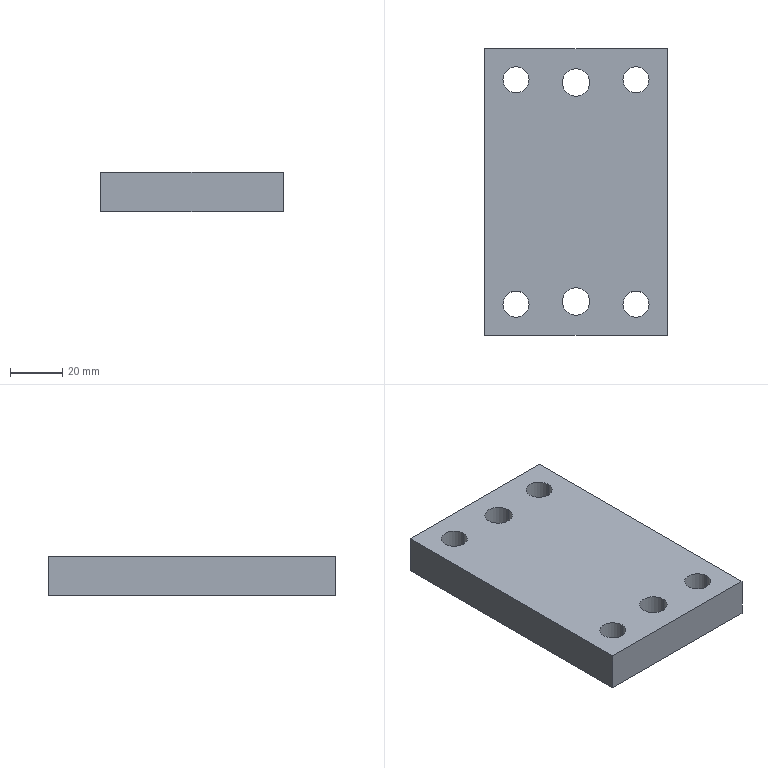Part | STEP file | Part 9^超升波生产线-2 | 1 solid | 18 faces | box 70 x 110 x 15 mm | volume 108190 mm3 | cylinder 12 | plane 6 | commonest cylinder face diameters 10 x8 10.5 x4
STEP:
#1=CARTESIAN_POINT('',(18.,-43.,15.));
#2=VERTEX_POINT('',#1);
#3=CARTESIAN_POINT('',(28.,-43.,15.));
#4=VERTEX_POINT('',#3);
#5=CARTESIAN_POINT('',(23.,-43.,15.));
#6=DIRECTION('',(0.,0.,1.));
#7=DIRECTION('',(1.,0.,0.));
#8=AXIS2_PLACEMENT_3D('',#5,#6,#7);
#9=CIRCLE('',#8,5.);
#10=EDGE_CURVE('',#2,#4,#9,.T.);
#11=ORIENTED_EDGE('',*,*,#10,.T.);
#12=CARTESIAN_POINT('',(28.,-43.,0.));
#13=VERTEX_POINT('',#12);
#14=CARTESIAN_POINT('',(28.,-43.,15.));
#15=DIRECTION('',(0.,0.,-1.));
#16=VECTOR('',#15,1000.);
#17=LINE('',#14,#16);
#18=EDGE_CURVE('',#4,#13,#17,.T.);
#19=ORIENTED_EDGE('',*,*,#18,.T.);
#20=CARTESIAN_POINT('',(18.,-43.,0.));
#21=VERTEX_POINT('',#20);
#22=CARTESIAN_POINT('',(23.,-43.,0.));
#23=DIRECTION('',(0.,0.,1.));
#24=DIRECTION('',(1.,0.,0.));
#25=AXIS2_PLACEMENT_3D('',#22,#23,#24);
#26=CIRCLE('',#25,5.);
#27=EDGE_CURVE('',#21,#13,#26,.T.);
#28=ORIENTED_EDGE('',*,*,#27,.F.);
#29=CARTESIAN_POINT('',(18.,-43.,15.));
#30=DIRECTION('',(0.,0.,-1.));
#31=VECTOR('',#30,1000.);
#32=LINE('',#29,#31);
#33=EDGE_CURVE('',#2,#21,#32,.T.);
#34=ORIENTED_EDGE('',*,*,#33,.F.);
#35=EDGE_LOOP('',(#11,#19,#28,#34));
#36=FACE_OUTER_BOUND('',#35,.T.);
#37=CARTESIAN_POINT('',(23.,-43.,15.));
#38=DIRECTION('',(0.,0.,-1.));
#39=DIRECTION('',(-1.,0.,0.));
#40=AXIS2_PLACEMENT_3D('',#37,#38,#39);
#41=CYLINDRICAL_SURFACE('',#40,5.);
#42=ADVANCED_FACE('',(#36),#41,.F.);
#43=CARTESIAN_POINT('',(-28.,-43.,15.));
#44=VERTEX_POINT('',#43);
#45=CARTESIAN_POINT('',(-18.,-43.,15.));
#46=VERTEX_POINT('',#45);
#47=CARTESIAN_POINT('',(-23.,-43.,15.));
#48=DIRECTION('',(0.,0.,1.));
#49=DIRECTION('',(1.,0.,0.));
#50=AXIS2_PLACEMENT_3D('',#47,#48,#49);
#51=CIRCLE('',#50,5.);
#52=EDGE_CURVE('',#44,#46,#51,.T.);
#53=ORIENTED_EDGE('',*,*,#52,.T.);
#54=CARTESIAN_POINT('',(-18.,-43.,0.));
#55=VERTEX_POINT('',#54);
#56=CARTESIAN_POINT('',(-18.,-43.,15.));
#57=DIRECTION('',(0.,0.,-1.));
#58=VECTOR('',#57,1000.);
#59=LINE('',#56,#58);
#60=EDGE_CURVE('',#46,#55,#59,.T.);
#61=ORIENTED_EDGE('',*,*,#60,.T.);
#62=CARTESIAN_POINT('',(-28.,-43.,0.));
#63=VERTEX_POINT('',#62);
#64=CARTESIAN_POINT('',(-23.,-43.,0.));
#65=DIRECTION('',(0.,0.,1.));
#66=DIRECTION('',(1.,0.,0.));
#67=AXIS2_PLACEMENT_3D('',#64,#65,#66);
#68=CIRCLE('',#67,5.);
#69=EDGE_CURVE('',#63,#55,#68,.T.);
#70=ORIENTED_EDGE('',*,*,#69,.F.);
#71=CARTESIAN_POINT('',(-28.,-43.,15.));
#72=DIRECTION('',(0.,0.,-1.));
#73=VECTOR('',#72,1000.);
#74=LINE('',#71,#73);
#75=EDGE_CURVE('',#44,#63,#74,.T.);
#76=ORIENTED_EDGE('',*,*,#75,.F.);
#77=EDGE_LOOP('',(#53,#61,#70,#76));
#78=FACE_OUTER_BOUND('',#77,.T.);
#79=CARTESIAN_POINT('',(-23.,-43.,15.));
#80=DIRECTION('',(0.,0.,-1.));
#81=DIRECTION('',(-1.,0.,0.));
#82=AXIS2_PLACEMENT_3D('',#79,#80,#81);
#83=CYLINDRICAL_SURFACE('',#82,5.);
#84=ADVANCED_FACE('',(#78),#83,.F.);
#85=CARTESIAN_POINT('',(18.,43.,15.));
#86=VERTEX_POINT('',#85);
#87=CARTESIAN_POINT('',(28.,43.,15.));
#88=VERTEX_POINT('',#87);
#89=CARTESIAN_POINT('',(23.,43.,15.));
#90=DIRECTION('',(0.,0.,1.));
#91=DIRECTION('',(1.,0.,0.));
#92=AXIS2_PLACEMENT_3D('',#89,#90,#91);
#93=CIRCLE('',#92,5.);
#94=EDGE_CURVE('',#86,#88,#93,.T.);
#95=ORIENTED_EDGE('',*,*,#94,.T.);
#96=CARTESIAN_POINT('',(28.,43.,0.));
#97=VERTEX_POINT('',#96);
#98=CARTESIAN_POINT('',(28.,43.,15.));
#99=DIRECTION('',(0.,0.,-1.));
#100=VECTOR('',#99,1000.);
#101=LINE('',#98,#100);
#102=EDGE_CURVE('',#88,#97,#101,.T.);
#103=ORIENTED_EDGE('',*,*,#102,.T.);
#104=CARTESIAN_POINT('',(18.,43.,0.));
#105=VERTEX_POINT('',#104);
#106=CARTESIAN_POINT('',(23.,43.,0.));
#107=DIRECTION('',(0.,0.,1.));
#108=DIRECTION('',(1.,0.,0.));
#109=AXIS2_PLACEMENT_3D('',#106,#107,#108);
#110=CIRCLE('',#109,5.);
#111=EDGE_CURVE('',#105,#97,#110,.T.);
#112=ORIENTED_EDGE('',*,*,#111,.F.);
#113=CARTESIAN_POINT('',(18.,43.,15.));
#114=DIRECTION('',(0.,0.,-1.));
#115=VECTOR('',#114,1000.);
#116=LINE('',#113,#115);
#117=EDGE_CURVE('',#86,#105,#116,.T.);
#118=ORIENTED_EDGE('',*,*,#117,.F.);
#119=EDGE_LOOP('',(#95,#103,#112,#118));
#120=FACE_OUTER_BOUND('',#119,.T.);
#121=CARTESIAN_POINT('',(23.,43.,15.));
#122=DIRECTION('',(0.,0.,-1.));
#123=DIRECTION('',(-1.,0.,0.));
#124=AXIS2_PLACEMENT_3D('',#121,#122,#123);
#125=CYLINDRICAL_SURFACE('',#124,5.);
#126=ADVANCED_FACE('',(#120),#125,.F.);
#127=CARTESIAN_POINT('',(-28.,43.,15.));
#128=VERTEX_POINT('',#127);
#129=CARTESIAN_POINT('',(-18.,43.,15.));
#130=VERTEX_POINT('',#129);
#131=CARTESIAN_POINT('',(-23.,43.,15.));
#132=DIRECTION('',(0.,0.,1.));
#133=DIRECTION('',(1.,0.,0.));
#134=AXIS2_PLACEMENT_3D('',#131,#132,#133);
#135=CIRCLE('',#134,5.);
#136=EDGE_CURVE('',#128,#130,#135,.T.);
#137=ORIENTED_EDGE('',*,*,#136,.T.);
#138=CARTESIAN_POINT('',(-18.,43.,0.));
#139=VERTEX_POINT('',#138);
#140=CARTESIAN_POINT('',(-18.,43.,15.));
#141=DIRECTION('',(0.,0.,-1.));
#142=VECTOR('',#141,1000.);
#143=LINE('',#140,#142);
#144=EDGE_CURVE('',#130,#139,#143,.T.);
#145=ORIENTED_EDGE('',*,*,#144,.T.);
#146=CARTESIAN_POINT('',(-28.,43.,0.));
#147=VERTEX_POINT('',#146);
#148=CARTESIAN_POINT('',(-23.,43.,0.));
#149=DIRECTION('',(0.,0.,1.));
#150=DIRECTION('',(1.,0.,0.));
#151=AXIS2_PLACEMENT_3D('',#148,#149,#150);
#152=CIRCLE('',#151,5.);
#153=EDGE_CURVE('',#147,#139,#152,.T.);
#154=ORIENTED_EDGE('',*,*,#153,.F.);
#155=CARTESIAN_POINT('',(-28.,43.,15.));
#156=DIRECTION('',(0.,0.,-1.));
#157=VECTOR('',#156,1000.);
#158=LINE('',#155,#157);
#159=EDGE_CURVE('',#128,#147,#158,.T.);
#160=ORIENTED_EDGE('',*,*,#159,.F.);
#161=EDGE_LOOP('',(#137,#145,#154,#160));
#162=FACE_OUTER_BOUND('',#161,.T.);
#163=CARTESIAN_POINT('',(-23.,43.,15.));
#164=DIRECTION('',(0.,0.,-1.));
#165=DIRECTION('',(-1.,0.,0.));
#166=AXIS2_PLACEMENT_3D('',#163,#164,#165);
#167=CYLINDRICAL_SURFACE('',#166,5.);
#168=ADVANCED_FACE('',(#162),#167,.F.);
#169=CARTESIAN_POINT('',(-5.25,-42.,15.));
#170=VERTEX_POINT('',#169);
#171=CARTESIAN_POINT('',(5.25,-42.,15.));
#172=VERTEX_POINT('',#171);
#173=CARTESIAN_POINT('',(0.,-42.,15.));
#174=DIRECTION('',(0.,0.,1.));
#175=DIRECTION('',(1.,0.,0.));
#176=AXIS2_PLACEMENT_3D('',#173,#174,#175);
#177=CIRCLE('',#176,5.25);
#178=EDGE_CURVE('',#170,#172,#177,.T.);
#179=ORIENTED_EDGE('',*,*,#178,.T.);
#180=CARTESIAN_POINT('',(5.25,-42.,0.));
#181=VERTEX_POINT('',#180);
#182=CARTESIAN_POINT('',(5.25,-42.,15.));
#183=DIRECTION('',(0.,0.,-1.));
#184=VECTOR('',#183,1000.);
#185=LINE('',#182,#184);
#186=EDGE_CURVE('',#172,#181,#185,.T.);
#187=ORIENTED_EDGE('',*,*,#186,.T.);
#188=CARTESIAN_POINT('',(-5.25,-42.,0.));
#189=VERTEX_POINT('',#188);
#190=CARTESIAN_POINT('',(0.,-42.,0.));
#191=DIRECTION('',(0.,0.,1.));
#192=DIRECTION('',(1.,0.,0.));
#193=AXIS2_PLACEMENT_3D('',#190,#191,#192);
#194=CIRCLE('',#193,5.25);
#195=EDGE_CURVE('',#189,#181,#194,.T.);
#196=ORIENTED_EDGE('',*,*,#195,.F.);
#197=CARTESIAN_POINT('',(-5.25,-42.,15.));
#198=DIRECTION('',(0.,0.,-1.));
#199=VECTOR('',#198,1000.);
#200=LINE('',#197,#199);
#201=EDGE_CURVE('',#170,#189,#200,.T.);
#202=ORIENTED_EDGE('',*,*,#201,.F.);
#203=EDGE_LOOP('',(#179,#187,#196,#202));
#204=FACE_OUTER_BOUND('',#203,.T.);
#205=CARTESIAN_POINT('',(0.,-42.,15.));
#206=DIRECTION('',(0.,0.,-1.));
#207=DIRECTION('',(-1.,0.,0.));
#208=AXIS2_PLACEMENT_3D('',#205,#206,#207);
#209=CYLINDRICAL_SURFACE('',#208,5.25);
#210=ADVANCED_FACE('',(#204),#209,.F.);
#211=CARTESIAN_POINT('',(-5.25,42.,15.));
#212=VERTEX_POINT('',#211);
#213=CARTESIAN_POINT('',(5.25,42.,15.));
#214=VERTEX_POINT('',#213);
#215=CARTESIAN_POINT('',(0.,42.,15.));
#216=DIRECTION('',(0.,0.,1.));
#217=DIRECTION('',(1.,0.,0.));
#218=AXIS2_PLACEMENT_3D('',#215,#216,#217);
#219=CIRCLE('',#218,5.25);
#220=EDGE_CURVE('',#212,#214,#219,.T.);
#221=ORIENTED_EDGE('',*,*,#220,.T.);
#222=CARTESIAN_POINT('',(5.25,42.,0.));
#223=VERTEX_POINT('',#222);
#224=CARTESIAN_POINT('',(5.25,42.,15.));
#225=DIRECTION('',(0.,0.,-1.));
#226=VECTOR('',#225,1000.);
#227=LINE('',#224,#226);
#228=EDGE_CURVE('',#214,#223,#227,.T.);
#229=ORIENTED_EDGE('',*,*,#228,.T.);
#230=CARTESIAN_POINT('',(-5.25,42.,0.));
#231=VERTEX_POINT('',#230);
#232=CARTESIAN_POINT('',(0.,42.,0.));
#233=DIRECTION('',(0.,0.,1.));
#234=DIRECTION('',(1.,0.,0.));
#235=AXIS2_PLACEMENT_3D('',#232,#233,#234);
#236=CIRCLE('',#235,5.25);
#237=EDGE_CURVE('',#231,#223,#236,.T.);
#238=ORIENTED_EDGE('',*,*,#237,.F.);
#239=CARTESIAN_POINT('',(-5.25,42.,15.));
#240=DIRECTION('',(0.,0.,-1.));
#241=VECTOR('',#240,1000.);
#242=LINE('',#239,#241);
#243=EDGE_CURVE('',#212,#231,#242,.T.);
#244=ORIENTED_EDGE('',*,*,#243,.F.);
#245=EDGE_LOOP('',(#221,#229,#238,#244));
#246=FACE_OUTER_BOUND('',#245,.T.);
#247=CARTESIAN_POINT('',(0.,42.,15.));
#248=DIRECTION('',(0.,0.,-1.));
#249=DIRECTION('',(-1.,0.,0.));
#250=AXIS2_PLACEMENT_3D('',#247,#248,#249);
#251=CYLINDRICAL_SURFACE('',#250,5.25);
#252=ADVANCED_FACE('',(#246),#251,.F.);
#253=ORIENTED_EDGE('',*,*,#52,.F.);
#254=CARTESIAN_POINT('',(-23.,-43.,15.));
#255=DIRECTION('',(0.,0.,1.));
#256=DIRECTION('',(1.,0.,0.));
#257=AXIS2_PLACEMENT_3D('',#254,#255,#256);
#258=CIRCLE('',#257,5.);
#259=EDGE_CURVE('',#46,#44,#258,.T.);
#260=ORIENTED_EDGE('',*,*,#259,.F.);
#261=EDGE_LOOP('',(#253,#260));
#262=FACE_BOUND('',#261,.T.);
#263=ORIENTED_EDGE('',*,*,#136,.F.);
#264=CARTESIAN_POINT('',(-23.,43.,15.));
#265=DIRECTION('',(0.,0.,1.));
#266=DIRECTION('',(1.,0.,0.));
#267=AXIS2_PLACEMENT_3D('',#264,#265,#266);
#268=CIRCLE('',#267,5.);
#269=EDGE_CURVE('',#130,#128,#268,.T.);
#270=ORIENTED_EDGE('',*,*,#269,.F.);
#271=EDGE_LOOP('',(#263,#270));
#272=FACE_BOUND('',#271,.T.);
#273=ORIENTED_EDGE('',*,*,#220,.F.);
#274=CARTESIAN_POINT('',(0.,42.,15.));
#275=DIRECTION('',(0.,0.,1.));
#276=DIRECTION('',(1.,0.,0.));
#277=AXIS2_PLACEMENT_3D('',#274,#275,#276);
#278=CIRCLE('',#277,5.25);
#279=EDGE_CURVE('',#214,#212,#278,.T.);
#280=ORIENTED_EDGE('',*,*,#279,.F.);
#281=EDGE_LOOP('',(#273,#280));
#282=FACE_BOUND('',#281,.T.);
#283=CARTESIAN_POINT('',(35.,-55.,15.));
#284=VERTEX_POINT('',#283);
#285=CARTESIAN_POINT('',(35.,55.,15.));
#286=VERTEX_POINT('',#285);
#287=CARTESIAN_POINT('',(35.,55.,15.));
#288=DIRECTION('',(0.,1.,0.));
#289=VECTOR('',#288,1000.);
#290=LINE('',#287,#289);
#291=EDGE_CURVE('',#284,#286,#290,.T.);
#292=ORIENTED_EDGE('',*,*,#291,.T.);
#293=CARTESIAN_POINT('',(-35.,55.,15.));
#294=VERTEX_POINT('',#293);
#295=CARTESIAN_POINT('',(-35.,55.,15.));
#296=DIRECTION('',(-1.,0.,0.));
#297=VECTOR('',#296,1000.);
#298=LINE('',#295,#297);
#299=EDGE_CURVE('',#286,#294,#298,.T.);
#300=ORIENTED_EDGE('',*,*,#299,.T.);
#301=CARTESIAN_POINT('',(-35.,-55.,15.));
#302=VERTEX_POINT('',#301);
#303=CARTESIAN_POINT('',(-35.,55.,15.));
#304=DIRECTION('',(0.,-1.,0.));
#305=VECTOR('',#304,1000.);
#306=LINE('',#303,#305);
#307=EDGE_CURVE('',#294,#302,#306,.T.);
#308=ORIENTED_EDGE('',*,*,#307,.T.);
#309=CARTESIAN_POINT('',(-35.,-55.,15.));
#310=DIRECTION('',(1.,0.,0.));
#311=VECTOR('',#310,1000.);
#312=LINE('',#309,#311);
#313=EDGE_CURVE('',#302,#284,#312,.T.);
#314=ORIENTED_EDGE('',*,*,#313,.T.);
#315=EDGE_LOOP('',(#292,#300,#308,#314));
#316=FACE_OUTER_BOUND('',#315,.T.);
#317=ORIENTED_EDGE('',*,*,#178,.F.);
#318=CARTESIAN_POINT('',(0.,-42.,15.));
#319=DIRECTION('',(0.,0.,1.));
#320=DIRECTION('',(1.,0.,0.));
#321=AXIS2_PLACEMENT_3D('',#318,#319,#320);
#322=CIRCLE('',#321,5.25);
#323=EDGE_CURVE('',#172,#170,#322,.T.);
#324=ORIENTED_EDGE('',*,*,#323,.F.);
#325=EDGE_LOOP('',(#317,#324));
#326=FACE_BOUND('',#325,.T.);
#327=ORIENTED_EDGE('',*,*,#94,.F.);
#328=CARTESIAN_POINT('',(23.,43.,15.));
#329=DIRECTION('',(0.,0.,1.));
#330=DIRECTION('',(1.,0.,0.));
#331=AXIS2_PLACEMENT_3D('',#328,#329,#330);
#332=CIRCLE('',#331,5.);
#333=EDGE_CURVE('',#88,#86,#332,.T.);
#334=ORIENTED_EDGE('',*,*,#333,.F.);
#335=EDGE_LOOP('',(#327,#334));
#336=FACE_BOUND('',#335,.T.);
#337=ORIENTED_EDGE('',*,*,#10,.F.);
#338=CARTESIAN_POINT('',(23.,-43.,15.));
#339=DIRECTION('',(0.,0.,1.));
#340=DIRECTION('',(1.,0.,0.));
#341=AXIS2_PLACEMENT_3D('',#338,#339,#340);
#342=CIRCLE('',#341,5.);
#343=EDGE_CURVE('',#4,#2,#342,.T.);
#344=ORIENTED_EDGE('',*,*,#343,.F.);
#345=EDGE_LOOP('',(#337,#344));
#346=FACE_BOUND('',#345,.T.);
#347=CARTESIAN_POINT('',(35.,-55.,15.));
#348=DIRECTION('',(0.,0.,1.));
#349=DIRECTION('',(1.,0.,0.));
#350=AXIS2_PLACEMENT_3D('',#347,#348,#349);
#351=PLANE('',#350);
#352=ADVANCED_FACE('',(#262,#272,#282,#316,#326,#336,#346),#351,.T.);
#353=ORIENTED_EDGE('',*,*,#69,.T.);
#354=CARTESIAN_POINT('',(-23.,-43.,0.));
#355=DIRECTION('',(0.,0.,1.));
#356=DIRECTION('',(1.,0.,0.));
#357=AXIS2_PLACEMENT_3D('',#354,#355,#356);
#358=CIRCLE('',#357,5.);
#359=EDGE_CURVE('',#55,#63,#358,.T.);
#360=ORIENTED_EDGE('',*,*,#359,.T.);
#361=EDGE_LOOP('',(#353,#360));
#362=FACE_BOUND('',#361,.T.);
#363=ORIENTED_EDGE('',*,*,#153,.T.);
#364=CARTESIAN_POINT('',(-23.,43.,0.));
#365=DIRECTION('',(0.,0.,1.));
#366=DIRECTION('',(1.,0.,0.));
#367=AXIS2_PLACEMENT_3D('',#364,#365,#366);
#368=CIRCLE('',#367,5.);
#369=EDGE_CURVE('',#139,#147,#368,.T.);
#370=ORIENTED_EDGE('',*,*,#369,.T.);
#371=EDGE_LOOP('',(#363,#370));
#372=FACE_BOUND('',#371,.T.);
#373=ORIENTED_EDGE('',*,*,#237,.T.);
#374=CARTESIAN_POINT('',(0.,42.,0.));
#375=DIRECTION('',(0.,0.,1.));
#376=DIRECTION('',(1.,0.,0.));
#377=AXIS2_PLACEMENT_3D('',#374,#375,#376);
#378=CIRCLE('',#377,5.25);
#379=EDGE_CURVE('',#223,#231,#378,.T.);
#380=ORIENTED_EDGE('',*,*,#379,.T.);
#381=EDGE_LOOP('',(#373,#380));
#382=FACE_BOUND('',#381,.T.);
#383=CARTESIAN_POINT('',(35.,-55.,0.));
#384=VERTEX_POINT('',#383);
#385=CARTESIAN_POINT('',(35.,55.,0.));
#386=VERTEX_POINT('',#385);
#387=CARTESIAN_POINT('',(35.,55.,0.));
#388=DIRECTION('',(0.,1.,0.));
#389=VECTOR('',#388,1000.);
#390=LINE('',#387,#389);
#391=EDGE_CURVE('',#384,#386,#390,.T.);
#392=ORIENTED_EDGE('',*,*,#391,.F.);
#393=CARTESIAN_POINT('',(-35.,-55.,0.));
#394=VERTEX_POINT('',#393);
#395=CARTESIAN_POINT('',(-35.,-55.,0.));
#396=DIRECTION('',(1.,0.,0.));
#397=VECTOR('',#396,1000.);
#398=LINE('',#395,#397);
#399=EDGE_CURVE('',#394,#384,#398,.T.);
#400=ORIENTED_EDGE('',*,*,#399,.F.);
#401=CARTESIAN_POINT('',(-35.,55.,0.));
#402=VERTEX_POINT('',#401);
#403=CARTESIAN_POINT('',(-35.,55.,0.));
#404=DIRECTION('',(0.,-1.,0.));
#405=VECTOR('',#404,1000.);
#406=LINE('',#403,#405);
#407=EDGE_CURVE('',#402,#394,#406,.T.);
#408=ORIENTED_EDGE('',*,*,#407,.F.);
#409=CARTESIAN_POINT('',(-35.,55.,0.));
#410=DIRECTION('',(-1.,0.,0.));
#411=VECTOR('',#410,1000.);
#412=LINE('',#409,#411);
#413=EDGE_CURVE('',#386,#402,#412,.T.);
#414=ORIENTED_EDGE('',*,*,#413,.F.);
#415=EDGE_LOOP('',(#392,#400,#408,#414));
#416=FACE_OUTER_BOUND('',#415,.T.);
#417=ORIENTED_EDGE('',*,*,#195,.T.);
#418=CARTESIAN_POINT('',(0.,-42.,0.));
#419=DIRECTION('',(0.,0.,1.));
#420=DIRECTION('',(1.,0.,0.));
#421=AXIS2_PLACEMENT_3D('',#418,#419,#420);
#422=CIRCLE('',#421,5.25);
#423=EDGE_CURVE('',#181,#189,#422,.T.);
#424=ORIENTED_EDGE('',*,*,#423,.T.);
#425=EDGE_LOOP('',(#417,#424));
#426=FACE_BOUND('',#425,.T.);
#427=ORIENTED_EDGE('',*,*,#111,.T.);
#428=CARTESIAN_POINT('',(23.,43.,0.));
#429=DIRECTION('',(0.,0.,1.));
#430=DIRECTION('',(1.,0.,0.));
#431=AXIS2_PLACEMENT_3D('',#428,#429,#430);
#432=CIRCLE('',#431,5.);
#433=EDGE_CURVE('',#97,#105,#432,.T.);
#434=ORIENTED_EDGE('',*,*,#433,.T.);
#435=EDGE_LOOP('',(#427,#434));
#436=FACE_BOUND('',#435,.T.);
#437=ORIENTED_EDGE('',*,*,#27,.T.);
#438=CARTESIAN_POINT('',(23.,-43.,0.));
#439=DIRECTION('',(0.,0.,1.));
#440=DIRECTION('',(1.,0.,0.));
#441=AXIS2_PLACEMENT_3D('',#438,#439,#440);
#442=CIRCLE('',#441,5.);
#443=EDGE_CURVE('',#13,#21,#442,.T.);
#444=ORIENTED_EDGE('',*,*,#443,.T.);
#445=EDGE_LOOP('',(#437,#444));
#446=FACE_BOUND('',#445,.T.);
#447=CARTESIAN_POINT('',(35.,-55.,0.));
#448=DIRECTION('',(0.,0.,1.));
#449=DIRECTION('',(1.,0.,0.));
#450=AXIS2_PLACEMENT_3D('',#447,#448,#449);
#451=PLANE('',#450);
#452=ADVANCED_FACE('',(#362,#372,#382,#416,#426,#436,#446),#451,.F.);
#453=ORIENTED_EDGE('',*,*,#391,.T.);
#454=CARTESIAN_POINT('',(35.,55.,15.));
#455=DIRECTION('',(0.,0.,-1.));
#456=VECTOR('',#455,1000.);
#457=LINE('',#454,#456);
#458=EDGE_CURVE('',#286,#386,#457,.T.);
#459=ORIENTED_EDGE('',*,*,#458,.F.);
#460=ORIENTED_EDGE('',*,*,#291,.F.);
#461=CARTESIAN_POINT('',(35.,-55.,15.));
#462=DIRECTION('',(0.,0.,-1.));
#463=VECTOR('',#462,1000.);
#464=LINE('',#461,#463);
#465=EDGE_CURVE('',#284,#384,#464,.T.);
#466=ORIENTED_EDGE('',*,*,#465,.T.);
#467=EDGE_LOOP('',(#453,#459,#460,#466));
#468=FACE_OUTER_BOUND('',#467,.T.);
#469=CARTESIAN_POINT('',(35.,55.,15.));
#470=DIRECTION('',(-1.,0.,0.));
#471=DIRECTION('',(0.,-1.,0.));
#472=AXIS2_PLACEMENT_3D('',#469,#470,#471);
#473=PLANE('',#472);
#474=ADVANCED_FACE('',(#468),#473,.F.);
#475=ORIENTED_EDGE('',*,*,#413,.T.);
#476=CARTESIAN_POINT('',(-35.,55.,15.));
#477=DIRECTION('',(0.,0.,-1.));
#478=VECTOR('',#477,1000.);
#479=LINE('',#476,#478);
#480=EDGE_CURVE('',#294,#402,#479,.T.);
#481=ORIENTED_EDGE('',*,*,#480,.F.);
#482=ORIENTED_EDGE('',*,*,#299,.F.);
#483=ORIENTED_EDGE('',*,*,#458,.T.);
#484=EDGE_LOOP('',(#475,#481,#482,#483));
#485=FACE_OUTER_BOUND('',#484,.T.);
#486=CARTESIAN_POINT('',(-35.,55.,15.));
#487=DIRECTION('',(0.,-1.,0.));
#488=DIRECTION('',(0.,0.,-1.));
#489=AXIS2_PLACEMENT_3D('',#486,#487,#488);
#490=PLANE('',#489);
#491=ADVANCED_FACE('',(#485),#490,.F.);
#492=ORIENTED_EDGE('',*,*,#407,.T.);
#493=CARTESIAN_POINT('',(-35.,-55.,15.));
#494=DIRECTION('',(0.,0.,-1.));
#495=VECTOR('',#494,1000.);
#496=LINE('',#493,#495);
#497=EDGE_CURVE('',#302,#394,#496,.T.);
#498=ORIENTED_EDGE('',*,*,#497,.F.);
#499=ORIENTED_EDGE('',*,*,#307,.F.);
#500=ORIENTED_EDGE('',*,*,#480,.T.);
#501=EDGE_LOOP('',(#492,#498,#499,#500));
#502=FACE_OUTER_BOUND('',#501,.T.);
#503=CARTESIAN_POINT('',(-35.,55.,15.));
#504=DIRECTION('',(1.,0.,0.));
#505=DIRECTION('',(0.,1.,0.));
#506=AXIS2_PLACEMENT_3D('',#503,#504,#505);
#507=PLANE('',#506);
#508=ADVANCED_FACE('',(#502),#507,.F.);
#509=ORIENTED_EDGE('',*,*,#399,.T.);
#510=ORIENTED_EDGE('',*,*,#465,.F.);
#511=ORIENTED_EDGE('',*,*,#313,.F.);
#512=ORIENTED_EDGE('',*,*,#497,.T.);
#513=EDGE_LOOP('',(#509,#510,#511,#512));
#514=FACE_OUTER_BOUND('',#513,.T.);
#515=CARTESIAN_POINT('',(-35.,-55.,15.));
#516=DIRECTION('',(0.,1.,0.));
#517=DIRECTION('',(0.,0.,1.));
#518=AXIS2_PLACEMENT_3D('',#515,#516,#517);
#519=PLANE('',#518);
#520=ADVANCED_FACE('',(#514),#519,.F.);
#521=ORIENTED_EDGE('',*,*,#228,.F.);
#522=ORIENTED_EDGE('',*,*,#279,.T.);
#523=ORIENTED_EDGE('',*,*,#243,.T.);
#524=ORIENTED_EDGE('',*,*,#379,.F.);
#525=EDGE_LOOP('',(#521,#522,#523,#524));
#526=FACE_OUTER_BOUND('',#525,.T.);
#527=CARTESIAN_POINT('',(0.,42.,15.));
#528=DIRECTION('',(0.,0.,-1.));
#529=DIRECTION('',(-1.,0.,0.));
#530=AXIS2_PLACEMENT_3D('',#527,#528,#529);
#531=CYLINDRICAL_SURFACE('',#530,5.25);
#532=ADVANCED_FACE('',(#526),#531,.F.);
#533=ORIENTED_EDGE('',*,*,#186,.F.);
#534=ORIENTED_EDGE('',*,*,#323,.T.);
#535=ORIENTED_EDGE('',*,*,#201,.T.);
#536=ORIENTED_EDGE('',*,*,#423,.F.);
#537=EDGE_LOOP('',(#533,#534,#535,#536));
#538=FACE_OUTER_BOUND('',#537,.T.);
#539=CARTESIAN_POINT('',(0.,-42.,15.));
#540=DIRECTION('',(0.,0.,-1.));
#541=DIRECTION('',(-1.,0.,0.));
#542=AXIS2_PLACEMENT_3D('',#539,#540,#541);
#543=CYLINDRICAL_SURFACE('',#542,5.25);
#544=ADVANCED_FACE('',(#538),#543,.F.);
#545=ORIENTED_EDGE('',*,*,#144,.F.);
#546=ORIENTED_EDGE('',*,*,#269,.T.);
#547=ORIENTED_EDGE('',*,*,#159,.T.);
#548=ORIENTED_EDGE('',*,*,#369,.F.);
#549=EDGE_LOOP('',(#545,#546,#547,#548));
#550=FACE_OUTER_BOUND('',#549,.T.);
#551=CARTESIAN_POINT('',(-23.,43.,15.));
#552=DIRECTION('',(0.,0.,-1.));
#553=DIRECTION('',(-1.,0.,0.));
#554=AXIS2_PLACEMENT_3D('',#551,#552,#553);
#555=CYLINDRICAL_SURFACE('',#554,5.);
#556=ADVANCED_FACE('',(#550),#555,.F.);
#557=ORIENTED_EDGE('',*,*,#102,.F.);
#558=ORIENTED_EDGE('',*,*,#333,.T.);
#559=ORIENTED_EDGE('',*,*,#117,.T.);
#560=ORIENTED_EDGE('',*,*,#433,.F.);
#561=EDGE_LOOP('',(#557,#558,#559,#560));
#562=FACE_OUTER_BOUND('',#561,.T.);
#563=CARTESIAN_POINT('',(23.,43.,15.));
#564=DIRECTION('',(0.,0.,-1.));
#565=DIRECTION('',(-1.,0.,0.));
#566=AXIS2_PLACEMENT_3D('',#563,#564,#565);
#567=CYLINDRICAL_SURFACE('',#566,5.);
#568=ADVANCED_FACE('',(#562),#567,.F.);
#569=ORIENTED_EDGE('',*,*,#60,.F.);
#570=ORIENTED_EDGE('',*,*,#259,.T.);
#571=ORIENTED_EDGE('',*,*,#75,.T.);
#572=ORIENTED_EDGE('',*,*,#359,.F.);
#573=EDGE_LOOP('',(#569,#570,#571,#572));
#574=FACE_OUTER_BOUND('',#573,.T.);
#575=CARTESIAN_POINT('',(-23.,-43.,15.));
#576=DIRECTION('',(0.,0.,-1.));
#577=DIRECTION('',(-1.,0.,0.));
#578=AXIS2_PLACEMENT_3D('',#575,#576,#577);
#579=CYLINDRICAL_SURFACE('',#578,5.);
#580=ADVANCED_FACE('',(#574),#579,.F.);
#581=ORIENTED_EDGE('',*,*,#18,.F.);
#582=ORIENTED_EDGE('',*,*,#343,.T.);
#583=ORIENTED_EDGE('',*,*,#33,.T.);
#584=ORIENTED_EDGE('',*,*,#443,.F.);
#585=EDGE_LOOP('',(#581,#582,#583,#584));
#586=FACE_OUTER_BOUND('',#585,.T.);
#587=CARTESIAN_POINT('',(23.,-43.,15.));
#588=DIRECTION('',(0.,0.,-1.));
#589=DIRECTION('',(-1.,0.,0.));
#590=AXIS2_PLACEMENT_3D('',#587,#588,#589);
#591=CYLINDRICAL_SURFACE('',#590,5.);
#592=ADVANCED_FACE('',(#586),#591,.F.);
#593=CLOSED_SHELL('',(#42,#84,#126,#168,#210,#252,#352,#452,#474,#491,#508,#520,#532,#544,#556,#568,#580,#592));
#594=MANIFOLD_SOLID_BREP('',#593);
#595=CARTESIAN_POINT('',(0.,0.,0.));
#596=DIRECTION('',(0.,0.,1.));
#597=DIRECTION('',(1.,0.,0.));
#598=AXIS2_PLACEMENT_3D('',#595,#596,#597);
#599=(LENGTH_UNIT()NAMED_UNIT(*)SI_UNIT(.MILLI.,.METRE.));
#600=UNCERTAINTY_MEASURE_WITH_UNIT(LENGTH_MEASURE(0.00001),#599,'','');
#601=(NAMED_UNIT(*)PLANE_ANGLE_UNIT()SI_UNIT($,.RADIAN.));
#602=(NAMED_UNIT(*)SI_UNIT($,.STERADIAN.)SOLID_ANGLE_UNIT());
#603=(GEOMETRIC_REPRESENTATION_CONTEXT(3)GLOBAL_UNCERTAINTY_ASSIGNED_CONTEXT((#600))GLOBAL_UNIT_ASSIGNED_CONTEXT((#599,#601,#602))REPRESENTATION_CONTEXT('',''));
#604=ADVANCED_BREP_SHAPE_REPRESENTATION('',(#594,#598),#603);